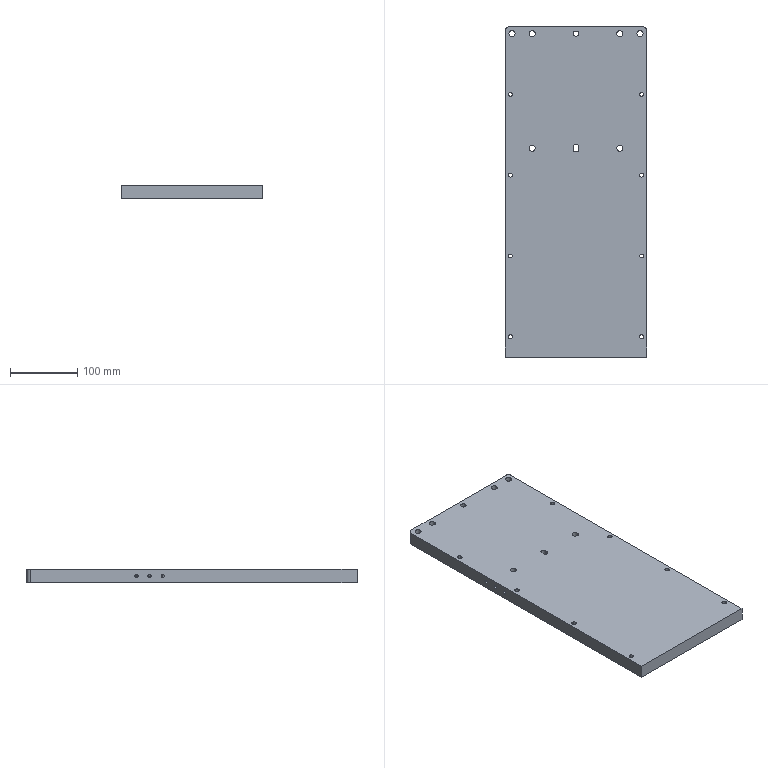Part | STEP file | KF-2212-050-007 | 1 solid | 106 faces | box 210 x 490 x 20 mm | volume 2037060 mm3 | cylinder 62 | cone 28 | plane 16 | commonest cylinder face diameters 6.6 x16 11 x16 5 x12 9 x12 8 x4 10 x2